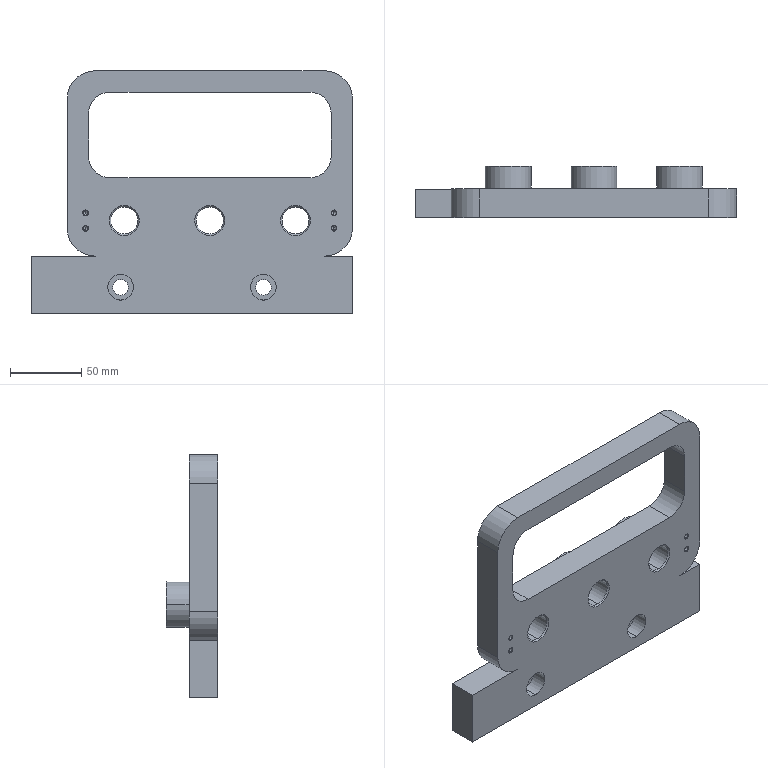Part | SolidWorks | features Fillet 4, ICE 4, Cut 3, HoleWzd 3, LPattern 3, 3DProfileFeature 2, Extrusion 1, Helix 1, SweepCut 1 | 1 solid | 120 faces | box 225 x 37.797 x 170 mm | volume 483949 mm3 | cylinder 60 | cone 26 | plane 25 | spline 9 | commonest cylinder face diameters 24 x24 3.3 x8 19 x6 32 x6 11 x4 18 x4